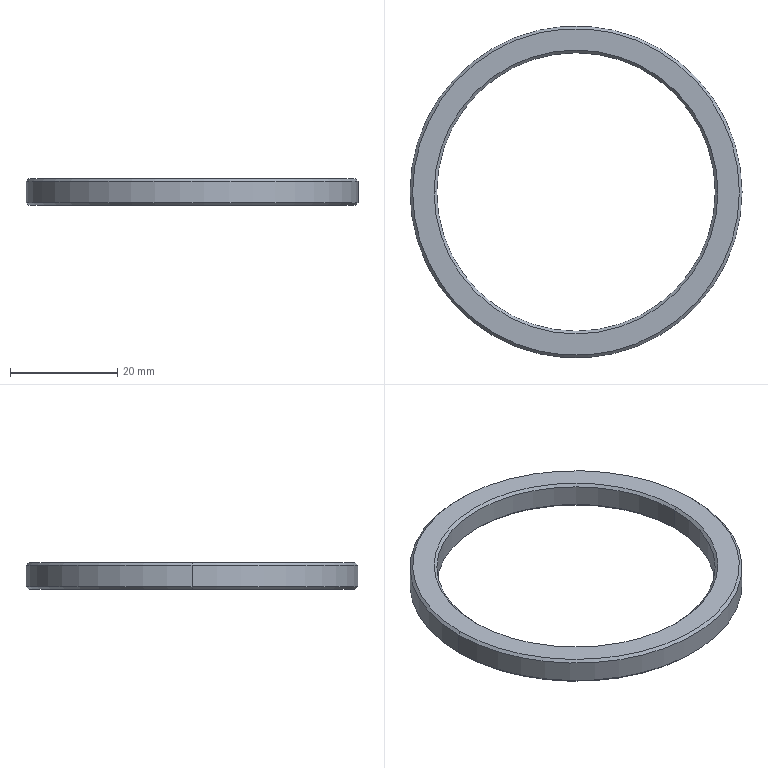Part | SolidWorks | features Chamfer 1, Extrusion 1 | 1 solid | 14 faces | box 62 x 62 x 5 mm | volume 4387 mm3 | cone 8 | cylinder 4 | plane 2 | commonest cylinder face diameters 52 x2 62 x2
STEP:
#1=CARTESIAN_POINT('',(30.5,0.,5.));
#2=VERTEX_POINT('',#1);
#3=CARTESIAN_POINT('',(-30.5,0.,5.));
#4=VERTEX_POINT('',#3);
#5=CARTESIAN_POINT('',(0.,0.,5.));
#6=DIRECTION('',(0.,0.,1.));
#7=DIRECTION('',(1.,0.,0.));
#8=AXIS2_PLACEMENT_3D('',#5,#6,#7);
#9=CIRCLE('',#8,30.5);
#10=EDGE_CURVE('',#2,#4,#9,.T.);
#11=ORIENTED_EDGE('',*,*,#10,.F.);
#12=CARTESIAN_POINT('',(31.,0.,4.5));
#13=VERTEX_POINT('',#12);
#14=CARTESIAN_POINT('',(30.5,0.,5.));
#15=DIRECTION('',(0.7071,0.,-0.7071));
#16=VECTOR('',#15,1000.);
#17=LINE('',#14,#16);
#18=EDGE_CURVE('',#2,#13,#17,.T.);
#19=ORIENTED_EDGE('',*,*,#18,.T.);
#20=CARTESIAN_POINT('',(-31.,0.,4.5));
#21=VERTEX_POINT('',#20);
#22=CARTESIAN_POINT('',(0.,0.,4.5));
#23=DIRECTION('',(0.,0.,-1.));
#24=DIRECTION('',(1.,0.,0.));
#25=AXIS2_PLACEMENT_3D('',#22,#23,#24);
#26=CIRCLE('',#25,31.);
#27=EDGE_CURVE('',#21,#13,#26,.T.);
#28=ORIENTED_EDGE('',*,*,#27,.F.);
#29=CARTESIAN_POINT('',(-30.5,0.,5.));
#30=DIRECTION('',(-0.7071,0.,-0.7071));
#31=VECTOR('',#30,1000.);
#32=LINE('',#29,#31);
#33=EDGE_CURVE('',#4,#21,#32,.T.);
#34=ORIENTED_EDGE('',*,*,#33,.F.);
#35=EDGE_LOOP('',(#11,#19,#28,#34));
#36=FACE_OUTER_BOUND('',#35,.T.);
#37=CARTESIAN_POINT('',(0.,0.,5.));
#38=DIRECTION('',(0.,0.,-1.));
#39=DIRECTION('',(-1.,0.,0.));
#40=AXIS2_PLACEMENT_3D('',#37,#38,#39);
#41=CONICAL_SURFACE('',#40,30.5,0.7854);
#42=ADVANCED_FACE('',(#36),#41,.T.);
#43=CARTESIAN_POINT('',(-26.,0.,4.5));
#44=VERTEX_POINT('',#43);
#45=CARTESIAN_POINT('',(26.,0.,4.5));
#46=VERTEX_POINT('',#45);
#47=CARTESIAN_POINT('',(0.,0.,4.5));
#48=DIRECTION('',(0.,0.,1.));
#49=DIRECTION('',(1.,0.,0.));
#50=AXIS2_PLACEMENT_3D('',#47,#48,#49);
#51=CIRCLE('',#50,26.);
#52=EDGE_CURVE('',#44,#46,#51,.T.);
#53=ORIENTED_EDGE('',*,*,#52,.F.);
#54=CARTESIAN_POINT('',(-26.5,0.,5.));
#55=VERTEX_POINT('',#54);
#56=CARTESIAN_POINT('',(-26.,0.,4.5));
#57=DIRECTION('',(-0.7071,0.,0.7071));
#58=VECTOR('',#57,1000.);
#59=LINE('',#56,#58);
#60=EDGE_CURVE('',#44,#55,#59,.T.);
#61=ORIENTED_EDGE('',*,*,#60,.T.);
#62=CARTESIAN_POINT('',(26.5,0.,5.));
#63=VERTEX_POINT('',#62);
#64=CARTESIAN_POINT('',(0.,0.,5.));
#65=DIRECTION('',(0.,0.,-1.));
#66=DIRECTION('',(1.,0.,0.));
#67=AXIS2_PLACEMENT_3D('',#64,#65,#66);
#68=CIRCLE('',#67,26.5);
#69=EDGE_CURVE('',#63,#55,#68,.T.);
#70=ORIENTED_EDGE('',*,*,#69,.F.);
#71=CARTESIAN_POINT('',(26.,0.,4.5));
#72=DIRECTION('',(0.7071,0.,0.7071));
#73=VECTOR('',#72,1000.);
#74=LINE('',#71,#73);
#75=EDGE_CURVE('',#46,#63,#74,.T.);
#76=ORIENTED_EDGE('',*,*,#75,.F.);
#77=EDGE_LOOP('',(#53,#61,#70,#76));
#78=FACE_OUTER_BOUND('',#77,.T.);
#79=CARTESIAN_POINT('',(0.,0.,4.5));
#80=DIRECTION('',(0.,0.,1.));
#81=DIRECTION('',(1.,0.,0.));
#82=AXIS2_PLACEMENT_3D('',#79,#80,#81);
#83=CONICAL_SURFACE('',#82,26.,0.7854);
#84=ADVANCED_FACE('',(#78),#83,.F.);
#85=CARTESIAN_POINT('',(-30.5,0.,0.));
#86=VERTEX_POINT('',#85);
#87=CARTESIAN_POINT('',(30.5,0.,0.));
#88=VERTEX_POINT('',#87);
#89=CARTESIAN_POINT('',(0.,0.,0.));
#90=DIRECTION('',(0.,0.,-1.));
#91=DIRECTION('',(1.,0.,0.));
#92=AXIS2_PLACEMENT_3D('',#89,#90,#91);
#93=CIRCLE('',#92,30.5);
#94=EDGE_CURVE('',#86,#88,#93,.T.);
#95=ORIENTED_EDGE('',*,*,#94,.F.);
#96=CARTESIAN_POINT('',(-31.,0.,0.5));
#97=VERTEX_POINT('',#96);
#98=CARTESIAN_POINT('',(-31.,0.,0.5));
#99=DIRECTION('',(-0.7071,0.,0.7071));
#100=VECTOR('',#99,1000.);
#101=LINE('',#98,#100);
#102=EDGE_CURVE('',#86,#97,#101,.T.);
#103=ORIENTED_EDGE('',*,*,#102,.T.);
#104=CARTESIAN_POINT('',(31.,0.,0.5));
#105=VERTEX_POINT('',#104);
#106=CARTESIAN_POINT('',(0.,0.,0.5));
#107=DIRECTION('',(0.,0.,1.));
#108=DIRECTION('',(1.,0.,0.));
#109=AXIS2_PLACEMENT_3D('',#106,#107,#108);
#110=CIRCLE('',#109,31.);
#111=EDGE_CURVE('',#105,#97,#110,.T.);
#112=ORIENTED_EDGE('',*,*,#111,.F.);
#113=CARTESIAN_POINT('',(31.,0.,0.5));
#114=DIRECTION('',(0.7071,0.,0.7071));
#115=VECTOR('',#114,1000.);
#116=LINE('',#113,#115);
#117=EDGE_CURVE('',#88,#105,#116,.T.);
#118=ORIENTED_EDGE('',*,*,#117,.F.);
#119=EDGE_LOOP('',(#95,#103,#112,#118));
#120=FACE_OUTER_BOUND('',#119,.T.);
#121=CARTESIAN_POINT('',(0.,0.,0.5));
#122=DIRECTION('',(0.,0.,1.));
#123=DIRECTION('',(1.,0.,0.));
#124=AXIS2_PLACEMENT_3D('',#121,#122,#123);
#125=CONICAL_SURFACE('',#124,31.,0.7854);
#126=ADVANCED_FACE('',(#120),#125,.T.);
#127=CARTESIAN_POINT('',(26.,0.,0.5));
#128=VERTEX_POINT('',#127);
#129=CARTESIAN_POINT('',(-26.,0.,0.5));
#130=VERTEX_POINT('',#129);
#131=CARTESIAN_POINT('',(0.,0.,0.5));
#132=DIRECTION('',(0.,0.,-1.));
#133=DIRECTION('',(1.,0.,0.));
#134=AXIS2_PLACEMENT_3D('',#131,#132,#133);
#135=CIRCLE('',#134,26.);
#136=EDGE_CURVE('',#128,#130,#135,.T.);
#137=ORIENTED_EDGE('',*,*,#136,.F.);
#138=CARTESIAN_POINT('',(26.5,0.,0.));
#139=VERTEX_POINT('',#138);
#140=CARTESIAN_POINT('',(26.5,0.,0.));
#141=DIRECTION('',(0.7071,0.,-0.7071));
#142=VECTOR('',#141,1000.);
#143=LINE('',#140,#142);
#144=EDGE_CURVE('',#128,#139,#143,.T.);
#145=ORIENTED_EDGE('',*,*,#144,.T.);
#146=CARTESIAN_POINT('',(-26.5,0.,0.));
#147=VERTEX_POINT('',#146);
#148=CARTESIAN_POINT('',(0.,0.,0.));
#149=DIRECTION('',(0.,0.,1.));
#150=DIRECTION('',(1.,0.,0.));
#151=AXIS2_PLACEMENT_3D('',#148,#149,#150);
#152=CIRCLE('',#151,26.5);
#153=EDGE_CURVE('',#147,#139,#152,.T.);
#154=ORIENTED_EDGE('',*,*,#153,.F.);
#155=CARTESIAN_POINT('',(-26.5,0.,0.));
#156=DIRECTION('',(-0.7071,0.,-0.7071));
#157=VECTOR('',#156,1000.);
#158=LINE('',#155,#157);
#159=EDGE_CURVE('',#130,#147,#158,.T.);
#160=ORIENTED_EDGE('',*,*,#159,.F.);
#161=EDGE_LOOP('',(#137,#145,#154,#160));
#162=FACE_OUTER_BOUND('',#161,.T.);
#163=CARTESIAN_POINT('',(0.,0.,0.));
#164=DIRECTION('',(0.,0.,-1.));
#165=DIRECTION('',(-1.,0.,0.));
#166=AXIS2_PLACEMENT_3D('',#163,#164,#165);
#167=CONICAL_SURFACE('',#166,26.5,0.7854);
#168=ADVANCED_FACE('',(#162),#167,.F.);
#169=ORIENTED_EDGE('',*,*,#52,.T.);
#170=CARTESIAN_POINT('',(26.,0.,5.));
#171=DIRECTION('',(0.,0.,-1.));
#172=VECTOR('',#171,1000.);
#173=LINE('',#170,#172);
#174=EDGE_CURVE('',#46,#128,#173,.T.);
#175=ORIENTED_EDGE('',*,*,#174,.T.);
#176=ORIENTED_EDGE('',*,*,#136,.T.);
#177=CARTESIAN_POINT('',(-26.,0.,5.));
#178=DIRECTION('',(0.,0.,-1.));
#179=VECTOR('',#178,1000.);
#180=LINE('',#177,#179);
#181=EDGE_CURVE('',#44,#130,#180,.T.);
#182=ORIENTED_EDGE('',*,*,#181,.F.);
#183=EDGE_LOOP('',(#169,#175,#176,#182));
#184=FACE_OUTER_BOUND('',#183,.T.);
#185=CARTESIAN_POINT('',(0.,0.,5.));
#186=DIRECTION('',(0.,0.,-1.));
#187=DIRECTION('',(-1.,0.,0.));
#188=AXIS2_PLACEMENT_3D('',#185,#186,#187);
#189=CYLINDRICAL_SURFACE('',#188,26.);
#190=ADVANCED_FACE('',(#184),#189,.F.);
#191=ORIENTED_EDGE('',*,*,#27,.T.);
#192=CARTESIAN_POINT('',(31.,0.,5.));
#193=DIRECTION('',(0.,0.,-1.));
#194=VECTOR('',#193,1000.);
#195=LINE('',#192,#194);
#196=EDGE_CURVE('',#13,#105,#195,.T.);
#197=ORIENTED_EDGE('',*,*,#196,.T.);
#198=ORIENTED_EDGE('',*,*,#111,.T.);
#199=CARTESIAN_POINT('',(-31.,0.,5.));
#200=DIRECTION('',(0.,0.,-1.));
#201=VECTOR('',#200,1000.);
#202=LINE('',#199,#201);
#203=EDGE_CURVE('',#21,#97,#202,.T.);
#204=ORIENTED_EDGE('',*,*,#203,.F.);
#205=EDGE_LOOP('',(#191,#197,#198,#204));
#206=FACE_OUTER_BOUND('',#205,.T.);
#207=CARTESIAN_POINT('',(0.,0.,5.));
#208=DIRECTION('',(0.,0.,-1.));
#209=DIRECTION('',(-1.,0.,0.));
#210=AXIS2_PLACEMENT_3D('',#207,#208,#209);
#211=CYLINDRICAL_SURFACE('',#210,31.);
#212=ADVANCED_FACE('',(#206),#211,.T.);
#213=ORIENTED_EDGE('',*,*,#69,.T.);
#214=CARTESIAN_POINT('',(0.,0.,5.));
#215=DIRECTION('',(0.,0.,-1.));
#216=DIRECTION('',(1.,0.,0.));
#217=AXIS2_PLACEMENT_3D('',#214,#215,#216);
#218=CIRCLE('',#217,26.5);
#219=EDGE_CURVE('',#55,#63,#218,.T.);
#220=ORIENTED_EDGE('',*,*,#219,.T.);
#221=EDGE_LOOP('',(#213,#220));
#222=FACE_BOUND('',#221,.T.);
#223=CARTESIAN_POINT('',(0.,0.,5.));
#224=DIRECTION('',(0.,0.,1.));
#225=DIRECTION('',(1.,0.,0.));
#226=AXIS2_PLACEMENT_3D('',#223,#224,#225);
#227=CIRCLE('',#226,30.5);
#228=EDGE_CURVE('',#4,#2,#227,.T.);
#229=ORIENTED_EDGE('',*,*,#228,.T.);
#230=ORIENTED_EDGE('',*,*,#10,.T.);
#231=EDGE_LOOP('',(#229,#230));
#232=FACE_OUTER_BOUND('',#231,.T.);
#233=CARTESIAN_POINT('',(0.,0.,5.));
#234=DIRECTION('',(0.,0.,1.));
#235=DIRECTION('',(1.,0.,0.));
#236=AXIS2_PLACEMENT_3D('',#233,#234,#235);
#237=PLANE('',#236);
#238=ADVANCED_FACE('',(#222,#232),#237,.T.);
#239=ORIENTED_EDGE('',*,*,#153,.T.);
#240=CARTESIAN_POINT('',(0.,0.,0.));
#241=DIRECTION('',(0.,0.,1.));
#242=DIRECTION('',(1.,0.,0.));
#243=AXIS2_PLACEMENT_3D('',#240,#241,#242);
#244=CIRCLE('',#243,26.5);
#245=EDGE_CURVE('',#139,#147,#244,.T.);
#246=ORIENTED_EDGE('',*,*,#245,.T.);
#247=EDGE_LOOP('',(#239,#246));
#248=FACE_BOUND('',#247,.T.);
#249=CARTESIAN_POINT('',(0.,0.,0.));
#250=DIRECTION('',(0.,0.,-1.));
#251=DIRECTION('',(1.,0.,0.));
#252=AXIS2_PLACEMENT_3D('',#249,#250,#251);
#253=CIRCLE('',#252,30.5);
#254=EDGE_CURVE('',#88,#86,#253,.T.);
#255=ORIENTED_EDGE('',*,*,#254,.T.);
#256=ORIENTED_EDGE('',*,*,#94,.T.);
#257=EDGE_LOOP('',(#255,#256));
#258=FACE_OUTER_BOUND('',#257,.T.);
#259=CARTESIAN_POINT('',(0.,0.,0.));
#260=DIRECTION('',(0.,0.,1.));
#261=DIRECTION('',(1.,0.,0.));
#262=AXIS2_PLACEMENT_3D('',#259,#260,#261);
#263=PLANE('',#262);
#264=ADVANCED_FACE('',(#248,#258),#263,.F.);
#265=ORIENTED_EDGE('',*,*,#196,.F.);
#266=CARTESIAN_POINT('',(0.,0.,4.5));
#267=DIRECTION('',(0.,0.,-1.));
#268=DIRECTION('',(1.,0.,0.));
#269=AXIS2_PLACEMENT_3D('',#266,#267,#268);
#270=CIRCLE('',#269,31.);
#271=EDGE_CURVE('',#13,#21,#270,.T.);
#272=ORIENTED_EDGE('',*,*,#271,.T.);
#273=ORIENTED_EDGE('',*,*,#203,.T.);
#274=CARTESIAN_POINT('',(0.,0.,0.5));
#275=DIRECTION('',(0.,0.,1.));
#276=DIRECTION('',(1.,0.,0.));
#277=AXIS2_PLACEMENT_3D('',#274,#275,#276);
#278=CIRCLE('',#277,31.);
#279=EDGE_CURVE('',#97,#105,#278,.T.);
#280=ORIENTED_EDGE('',*,*,#279,.T.);
#281=EDGE_LOOP('',(#265,#272,#273,#280));
#282=FACE_OUTER_BOUND('',#281,.T.);
#283=CARTESIAN_POINT('',(0.,0.,5.));
#284=DIRECTION('',(0.,0.,-1.));
#285=DIRECTION('',(-1.,0.,0.));
#286=AXIS2_PLACEMENT_3D('',#283,#284,#285);
#287=CYLINDRICAL_SURFACE('',#286,31.);
#288=ADVANCED_FACE('',(#282),#287,.T.);
#289=ORIENTED_EDGE('',*,*,#174,.F.);
#290=CARTESIAN_POINT('',(0.,0.,4.5));
#291=DIRECTION('',(0.,0.,1.));
#292=DIRECTION('',(1.,0.,0.));
#293=AXIS2_PLACEMENT_3D('',#290,#291,#292);
#294=CIRCLE('',#293,26.);
#295=EDGE_CURVE('',#46,#44,#294,.T.);
#296=ORIENTED_EDGE('',*,*,#295,.T.);
#297=ORIENTED_EDGE('',*,*,#181,.T.);
#298=CARTESIAN_POINT('',(0.,0.,0.5));
#299=DIRECTION('',(0.,0.,-1.));
#300=DIRECTION('',(1.,0.,0.));
#301=AXIS2_PLACEMENT_3D('',#298,#299,#300);
#302=CIRCLE('',#301,26.);
#303=EDGE_CURVE('',#130,#128,#302,.T.);
#304=ORIENTED_EDGE('',*,*,#303,.T.);
#305=EDGE_LOOP('',(#289,#296,#297,#304));
#306=FACE_OUTER_BOUND('',#305,.T.);
#307=CARTESIAN_POINT('',(0.,0.,5.));
#308=DIRECTION('',(0.,0.,-1.));
#309=DIRECTION('',(-1.,0.,0.));
#310=AXIS2_PLACEMENT_3D('',#307,#308,#309);
#311=CYLINDRICAL_SURFACE('',#310,26.);
#312=ADVANCED_FACE('',(#306),#311,.F.);
#313=ORIENTED_EDGE('',*,*,#144,.F.);
#314=ORIENTED_EDGE('',*,*,#303,.F.);
#315=ORIENTED_EDGE('',*,*,#159,.T.);
#316=ORIENTED_EDGE('',*,*,#245,.F.);
#317=EDGE_LOOP('',(#313,#314,#315,#316));
#318=FACE_OUTER_BOUND('',#317,.T.);
#319=CARTESIAN_POINT('',(0.,0.,0.));
#320=DIRECTION('',(0.,0.,-1.));
#321=DIRECTION('',(-1.,0.,0.));
#322=AXIS2_PLACEMENT_3D('',#319,#320,#321);
#323=CONICAL_SURFACE('',#322,26.5,0.7854);
#324=ADVANCED_FACE('',(#318),#323,.F.);
#325=ORIENTED_EDGE('',*,*,#102,.F.);
#326=ORIENTED_EDGE('',*,*,#254,.F.);
#327=ORIENTED_EDGE('',*,*,#117,.T.);
#328=ORIENTED_EDGE('',*,*,#279,.F.);
#329=EDGE_LOOP('',(#325,#326,#327,#328));
#330=FACE_OUTER_BOUND('',#329,.T.);
#331=CARTESIAN_POINT('',(0.,0.,0.5));
#332=DIRECTION('',(0.,0.,1.));
#333=DIRECTION('',(1.,0.,0.));
#334=AXIS2_PLACEMENT_3D('',#331,#332,#333);
#335=CONICAL_SURFACE('',#334,31.,0.7854);
#336=ADVANCED_FACE('',(#330),#335,.T.);
#337=ORIENTED_EDGE('',*,*,#60,.F.);
#338=ORIENTED_EDGE('',*,*,#295,.F.);
#339=ORIENTED_EDGE('',*,*,#75,.T.);
#340=ORIENTED_EDGE('',*,*,#219,.F.);
#341=EDGE_LOOP('',(#337,#338,#339,#340));
#342=FACE_OUTER_BOUND('',#341,.T.);
#343=CARTESIAN_POINT('',(0.,0.,4.5));
#344=DIRECTION('',(0.,0.,1.));
#345=DIRECTION('',(1.,0.,0.));
#346=AXIS2_PLACEMENT_3D('',#343,#344,#345);
#347=CONICAL_SURFACE('',#346,26.,0.7854);
#348=ADVANCED_FACE('',(#342),#347,.F.);
#349=ORIENTED_EDGE('',*,*,#18,.F.);
#350=ORIENTED_EDGE('',*,*,#228,.F.);
#351=ORIENTED_EDGE('',*,*,#33,.T.);
#352=ORIENTED_EDGE('',*,*,#271,.F.);
#353=EDGE_LOOP('',(#349,#350,#351,#352));
#354=FACE_OUTER_BOUND('',#353,.T.);
#355=CARTESIAN_POINT('',(0.,0.,5.));
#356=DIRECTION('',(0.,0.,-1.));
#357=DIRECTION('',(-1.,0.,0.));
#358=AXIS2_PLACEMENT_3D('',#355,#356,#357);
#359=CONICAL_SURFACE('',#358,30.5,0.7854);
#360=ADVANCED_FACE('',(#354),#359,.T.);
#361=CLOSED_SHELL('',(#42,#84,#126,#168,#190,#212,#238,#264,#288,#312,#324,#336,#348,#360));
#362=MANIFOLD_SOLID_BREP('',#361);
#363=CARTESIAN_POINT('',(0.,0.,0.));
#364=DIRECTION('',(0.,0.,1.));
#365=DIRECTION('',(1.,0.,0.));
#366=AXIS2_PLACEMENT_3D('',#363,#364,#365);
#367=(LENGTH_UNIT()NAMED_UNIT(*)SI_UNIT(.MILLI.,.METRE.));
#368=UNCERTAINTY_MEASURE_WITH_UNIT(LENGTH_MEASURE(0.00001),#367,'','');
#369=(NAMED_UNIT(*)PLANE_ANGLE_UNIT()SI_UNIT($,.RADIAN.));
#370=(NAMED_UNIT(*)SI_UNIT($,.STERADIAN.)SOLID_ANGLE_UNIT());
#371=(GEOMETRIC_REPRESENTATION_CONTEXT(3)GLOBAL_UNCERTAINTY_ASSIGNED_CONTEXT((#368))GLOBAL_UNIT_ASSIGNED_CONTEXT((#367,#369,#370))REPRESENTATION_CONTEXT('',''));
#372=ADVANCED_BREP_SHAPE_REPRESENTATION('',(#362,#366),#371);